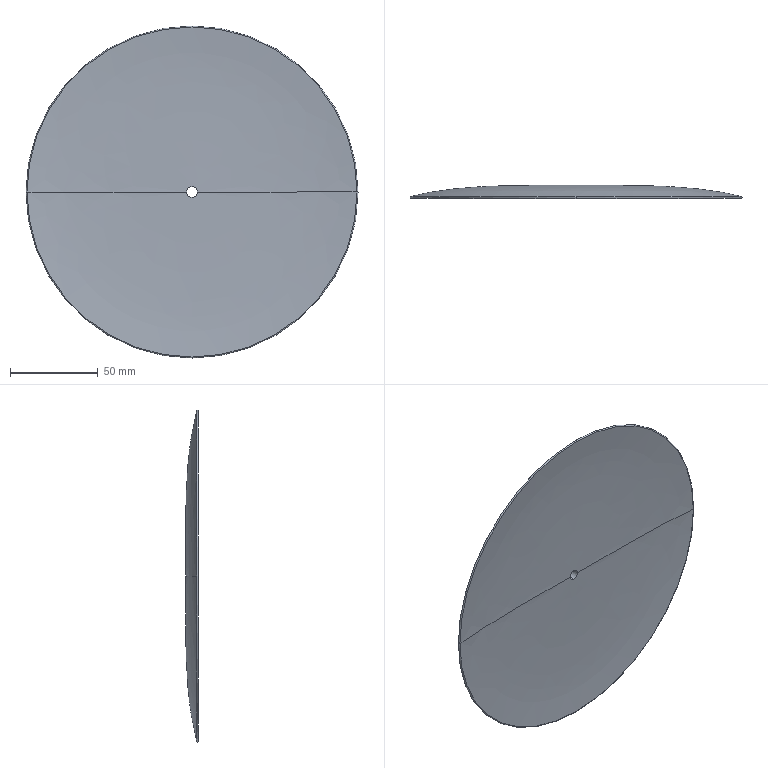Part | SolidWorks | features Fillet 1, ICE 1, Revolution 1 | 1 solid | 8 faces | box 189.61 x 7.325 x 189.61 mm | volume 102683 mm3 | spline 4 | cylinder 2 | torus 2 | commonest cylinder face diameters 6 x2
STEP:
#1=CARTESIAN_POINT('',(0.,-7.131,-94.253));
#2=VERTEX_POINT('',#1);
#3=CARTESIAN_POINT('',(94.253,-7.131,0.));
#4=VERTEX_POINT('',#3);
#5=CARTESIAN_POINT('',(0.,-7.131,0.));
#6=DIRECTION('',(0.,-1.,0.));
#7=DIRECTION('',(0.,0.,1.));
#8=AXIS2_PLACEMENT_3D('',#5,#6,#7);
#9=CIRCLE('',#8,94.253);
#10=EDGE_CURVE('',#2,#4,#9,.T.);
#11=ORIENTED_EDGE('',*,*,#10,.T.);
#12=CARTESIAN_POINT('',(3.,-4.995,0.));
#13=VERTEX_POINT('',#12);
#14=CARTESIAN_POINT('',(94.253,-7.131,0.));
#15=CARTESIAN_POINT('',(66.921,-4.289,0.));
#16=CARTESIAN_POINT('',(24.057,-4.927,0.));
#17=CARTESIAN_POINT('',(3.,-4.995,0.));
#18=B_SPLINE_CURVE_WITH_KNOTS('',3,(#14,#15,#16,#17),.UNSPECIFIED.,.F.,.F.,(4,4),(0.06526,0.9553),.UNSPECIFIED.);
#19=EDGE_CURVE('',#4,#13,#18,.T.);
#20=ORIENTED_EDGE('',*,*,#19,.T.);
#21=CARTESIAN_POINT('',(0.,-4.995,-3.));
#22=VERTEX_POINT('',#21);
#23=CARTESIAN_POINT('',(0.,-4.995,0.));
#24=DIRECTION('',(0.,-1.,0.));
#25=DIRECTION('',(0.,0.,1.));
#26=AXIS2_PLACEMENT_3D('',#23,#24,#25);
#27=CIRCLE('',#26,3.);
#28=EDGE_CURVE('',#22,#13,#27,.T.);
#29=ORIENTED_EDGE('',*,*,#28,.F.);
#30=CARTESIAN_POINT('',(-3.,-4.995,0.));
#31=VERTEX_POINT('',#30);
#32=CARTESIAN_POINT('',(0.,-4.995,0.));
#33=DIRECTION('',(0.,-1.,0.));
#34=DIRECTION('',(0.,0.,1.));
#35=AXIS2_PLACEMENT_3D('',#32,#33,#34);
#36=CIRCLE('',#35,3.);
#37=EDGE_CURVE('',#31,#22,#36,.T.);
#38=ORIENTED_EDGE('',*,*,#37,.F.);
#39=CARTESIAN_POINT('',(-94.253,-7.131,0.));
#40=VERTEX_POINT('',#39);
#41=CARTESIAN_POINT('',(-94.253,-7.131,0.));
#42=CARTESIAN_POINT('',(-66.921,-4.289,0.));
#43=CARTESIAN_POINT('',(-24.057,-4.927,0.));
#44=CARTESIAN_POINT('',(-3.,-4.995,0.));
#45=B_SPLINE_CURVE_WITH_KNOTS('',3,(#41,#42,#43,#44),.UNSPECIFIED.,.F.,.F.,(4,4),(0.06526,0.9553),.UNSPECIFIED.);
#46=EDGE_CURVE('',#40,#31,#45,.T.);
#47=ORIENTED_EDGE('',*,*,#46,.F.);
#48=CARTESIAN_POINT('',(0.,-7.131,0.));
#49=DIRECTION('',(0.,-1.,0.));
#50=DIRECTION('',(0.,0.,1.));
#51=AXIS2_PLACEMENT_3D('',#48,#49,#50);
#52=CIRCLE('',#51,94.253);
#53=EDGE_CURVE('',#40,#2,#52,.T.);
#54=ORIENTED_EDGE('',*,*,#53,.T.);
#55=EDGE_LOOP('',(#11,#20,#29,#38,#47,#54));
#56=FACE_OUTER_BOUND('',#55,.T.);
#57=CARTESIAN_POINT('',(94.253,-7.131,0.));
#58=CARTESIAN_POINT('',(94.253,-7.131,-188.507));
#59=CARTESIAN_POINT('',(-94.253,-7.131,-188.507));
#60=CARTESIAN_POINT('',(-94.253,-7.131,0.));
#61=CARTESIAN_POINT('',(66.921,-4.289,0.));
#62=CARTESIAN_POINT('',(66.921,-4.289,-133.842));
#63=CARTESIAN_POINT('',(-66.921,-4.289,-133.842));
#64=CARTESIAN_POINT('',(-66.921,-4.289,0.));
#65=CARTESIAN_POINT('',(24.057,-4.927,0.));
#66=CARTESIAN_POINT('',(24.057,-4.927,-48.114));
#67=CARTESIAN_POINT('',(-24.057,-4.927,-48.114));
#68=CARTESIAN_POINT('',(-24.057,-4.927,0.));
#69=CARTESIAN_POINT('',(3.,-4.995,0.));
#70=CARTESIAN_POINT('',(3.,-4.995,-6.));
#71=CARTESIAN_POINT('',(-3.,-4.995,-6.));
#72=CARTESIAN_POINT('',(-3.,-4.995,0.));
#73=(BOUNDED_SURFACE()B_SPLINE_SURFACE(3,3,((#57,#58,#59,#60),(#61,#62,#63,#64),(#65,#66,#67,#68),(#69,#70,#71,#72)),.UNSPECIFIED.,.F.,.F.,.F.)B_SPLINE_SURFACE_WITH_KNOTS((4,4),(4,4),(0.06526,0.9553),(0.,1.),.UNSPECIFIED.)GEOMETRIC_REPRESENTATION_ITEM()RATIONAL_B_SPLINE_SURFACE(((1.,0.3333,0.3333,1.),(1.,0.3333,0.3333,1.),(1.,0.3333,0.3333,1.),(1.,0.3333,0.3333,1.)))REPRESENTATION_ITEM('')SURFACE());
#74=ADVANCED_FACE('',(#56),#73,.T.);
#75=CARTESIAN_POINT('',(3.,0.01022,0.));
#76=VERTEX_POINT('',#75);
#77=CARTESIAN_POINT('',(0.,0.01022,-3.));
#78=VERTEX_POINT('',#77);
#79=CARTESIAN_POINT('',(0.,0.01022,0.));
#80=DIRECTION('',(0.,1.,0.));
#81=DIRECTION('',(0.,0.,1.));
#82=AXIS2_PLACEMENT_3D('',#79,#80,#81);
#83=CIRCLE('',#82,3.);
#84=EDGE_CURVE('',#76,#78,#83,.T.);
#85=ORIENTED_EDGE('',*,*,#84,.F.);
#86=CARTESIAN_POINT('',(94.435,-6.151,0.));
#87=VERTEX_POINT('',#86);
#88=CARTESIAN_POINT('',(3.,0.01022,0.));
#89=CARTESIAN_POINT('',(25.237,0.1482,0.));
#90=CARTESIAN_POINT('',(65.845,1.519,0.));
#91=CARTESIAN_POINT('',(94.435,-6.151,0.));
#92=B_SPLINE_CURVE_WITH_KNOTS('',3,(#88,#89,#90,#91),.UNSPECIFIED.,.F.,.F.,(4,4),(0.04205,0.94),.UNSPECIFIED.);
#93=EDGE_CURVE('',#76,#87,#92,.T.);
#94=ORIENTED_EDGE('',*,*,#93,.T.);
#95=CARTESIAN_POINT('',(0.,-6.151,-94.435));
#96=VERTEX_POINT('',#95);
#97=CARTESIAN_POINT('',(0.,-6.151,0.));
#98=DIRECTION('',(0.,1.,0.));
#99=DIRECTION('',(0.,0.,1.));
#100=AXIS2_PLACEMENT_3D('',#97,#98,#99);
#101=CIRCLE('',#100,94.435);
#102=EDGE_CURVE('',#87,#96,#101,.T.);
#103=ORIENTED_EDGE('',*,*,#102,.T.);
#104=CARTESIAN_POINT('',(-94.435,-6.151,0.));
#105=VERTEX_POINT('',#104);
#106=CARTESIAN_POINT('',(0.,-6.151,0.));
#107=DIRECTION('',(0.,1.,0.));
#108=DIRECTION('',(0.,0.,1.));
#109=AXIS2_PLACEMENT_3D('',#106,#107,#108);
#110=CIRCLE('',#109,94.435);
#111=EDGE_CURVE('',#96,#105,#110,.T.);
#112=ORIENTED_EDGE('',*,*,#111,.T.);
#113=CARTESIAN_POINT('',(-3.,0.01022,0.));
#114=VERTEX_POINT('',#113);
#115=CARTESIAN_POINT('',(-3.,0.01022,0.));
#116=CARTESIAN_POINT('',(-25.237,0.1482,0.));
#117=CARTESIAN_POINT('',(-65.845,1.519,0.));
#118=CARTESIAN_POINT('',(-94.435,-6.151,0.));
#119=B_SPLINE_CURVE_WITH_KNOTS('',3,(#115,#116,#117,#118),.UNSPECIFIED.,.F.,.F.,(4,4),(0.04205,0.94),.UNSPECIFIED.);
#120=EDGE_CURVE('',#114,#105,#119,.T.);
#121=ORIENTED_EDGE('',*,*,#120,.F.);
#122=CARTESIAN_POINT('',(0.,0.01022,0.));
#123=DIRECTION('',(0.,1.,0.));
#124=DIRECTION('',(0.,0.,1.));
#125=AXIS2_PLACEMENT_3D('',#122,#123,#124);
#126=CIRCLE('',#125,3.);
#127=EDGE_CURVE('',#78,#114,#126,.T.);
#128=ORIENTED_EDGE('',*,*,#127,.F.);
#129=EDGE_LOOP('',(#85,#94,#103,#112,#121,#128));
#130=FACE_OUTER_BOUND('',#129,.T.);
#131=CARTESIAN_POINT('',(3.,0.01022,0.));
#132=CARTESIAN_POINT('',(3.,0.01022,-6.));
#133=CARTESIAN_POINT('',(-3.,0.01022,-6.));
#134=CARTESIAN_POINT('',(-3.,0.01022,0.));
#135=CARTESIAN_POINT('',(25.237,0.1482,0.));
#136=CARTESIAN_POINT('',(25.237,0.1482,-50.474));
#137=CARTESIAN_POINT('',(-25.237,0.1482,-50.474));
#138=CARTESIAN_POINT('',(-25.237,0.1482,0.));
#139=CARTESIAN_POINT('',(65.845,1.519,0.));
#140=CARTESIAN_POINT('',(65.845,1.519,-131.691));
#141=CARTESIAN_POINT('',(-65.845,1.519,-131.691));
#142=CARTESIAN_POINT('',(-65.845,1.519,0.));
#143=CARTESIAN_POINT('',(94.435,-6.151,0.));
#144=CARTESIAN_POINT('',(94.435,-6.151,-188.869));
#145=CARTESIAN_POINT('',(-94.435,-6.151,-188.869));
#146=CARTESIAN_POINT('',(-94.435,-6.151,0.));
#147=(BOUNDED_SURFACE()B_SPLINE_SURFACE(3,3,((#131,#132,#133,#134),(#135,#136,#137,#138),(#139,#140,#141,#142),(#143,#144,#145,#146)),.UNSPECIFIED.,.F.,.F.,.F.)B_SPLINE_SURFACE_WITH_KNOTS((4,4),(4,4),(0.04205,0.94),(0.,1.),.UNSPECIFIED.)GEOMETRIC_REPRESENTATION_ITEM()RATIONAL_B_SPLINE_SURFACE(((1.,0.3333,0.3333,1.),(1.,0.3333,0.3333,1.),(1.,0.3333,0.3333,1.),(1.,0.3333,0.3333,1.)))REPRESENTATION_ITEM('')SURFACE());
#148=ADVANCED_FACE('',(#130),#147,.T.);
#149=CARTESIAN_POINT('',(0.,-4.995,3.));
#150=VERTEX_POINT('',#149);
#151=CARTESIAN_POINT('',(0.,-4.995,0.));
#152=DIRECTION('',(0.,-1.,0.));
#153=DIRECTION('',(0.,0.,1.));
#154=AXIS2_PLACEMENT_3D('',#151,#152,#153);
#155=CIRCLE('',#154,3.);
#156=EDGE_CURVE('',#150,#31,#155,.T.);
#157=ORIENTED_EDGE('',*,*,#156,.T.);
#158=ORIENTED_EDGE('',*,*,#37,.T.);
#159=CARTESIAN_POINT('',(0.,-23.,-3.));
#160=DIRECTION('',(0.,1.,0.));
#161=VECTOR('',#160,1000.);
#162=LINE('',#159,#161);
#163=EDGE_CURVE('',#22,#78,#162,.T.);
#164=ORIENTED_EDGE('',*,*,#163,.T.);
#165=ORIENTED_EDGE('',*,*,#127,.T.);
#166=CARTESIAN_POINT('',(0.,0.01022,3.));
#167=VERTEX_POINT('',#166);
#168=CARTESIAN_POINT('',(0.,0.01022,0.));
#169=DIRECTION('',(0.,1.,0.));
#170=DIRECTION('',(0.,0.,1.));
#171=AXIS2_PLACEMENT_3D('',#168,#169,#170);
#172=CIRCLE('',#171,3.);
#173=EDGE_CURVE('',#114,#167,#172,.T.);
#174=ORIENTED_EDGE('',*,*,#173,.T.);
#175=CARTESIAN_POINT('',(0.,-23.,3.));
#176=DIRECTION('',(0.,1.,0.));
#177=VECTOR('',#176,1000.);
#178=LINE('',#175,#177);
#179=EDGE_CURVE('',#150,#167,#178,.T.);
#180=ORIENTED_EDGE('',*,*,#179,.F.);
#181=EDGE_LOOP('',(#157,#158,#164,#165,#174,#180));
#182=FACE_OUTER_BOUND('',#181,.T.);
#183=CARTESIAN_POINT('',(0.,-23.,0.));
#184=DIRECTION('',(0.,1.,0.));
#185=DIRECTION('',(0.,0.,1.));
#186=AXIS2_PLACEMENT_3D('',#183,#184,#185);
#187=CYLINDRICAL_SURFACE('',#186,3.);
#188=ADVANCED_FACE('',(#182),#187,.F.);
#189=CARTESIAN_POINT('',(0.,-6.151,94.435));
#190=VERTEX_POINT('',#189);
#191=CARTESIAN_POINT('',(0.,-6.151,0.));
#192=DIRECTION('',(0.,1.,0.));
#193=DIRECTION('',(0.,0.,1.));
#194=AXIS2_PLACEMENT_3D('',#191,#192,#193);
#195=CIRCLE('',#194,94.435);
#196=EDGE_CURVE('',#190,#87,#195,.T.);
#197=ORIENTED_EDGE('',*,*,#196,.F.);
#198=CARTESIAN_POINT('',(0.,-7.131,94.253));
#199=VERTEX_POINT('',#198);
#200=CARTESIAN_POINT('',(0.,-6.634,94.305));
#201=DIRECTION('',(1.,0.,0.));
#202=DIRECTION('',(0.,0.,-1.));
#203=AXIS2_PLACEMENT_3D('',#200,#201,#202);
#204=CIRCLE('',#203,0.5);
#205=EDGE_CURVE('',#190,#199,#204,.T.);
#206=ORIENTED_EDGE('',*,*,#205,.T.);
#207=CARTESIAN_POINT('',(0.,-7.131,0.));
#208=DIRECTION('',(0.,-1.,0.));
#209=DIRECTION('',(0.,0.,1.));
#210=AXIS2_PLACEMENT_3D('',#207,#208,#209);
#211=CIRCLE('',#210,94.253);
#212=EDGE_CURVE('',#4,#199,#211,.T.);
#213=ORIENTED_EDGE('',*,*,#212,.F.);
#214=ORIENTED_EDGE('',*,*,#10,.F.);
#215=CARTESIAN_POINT('',(0.,-6.634,-94.305));
#216=DIRECTION('',(-1.,0.,0.));
#217=DIRECTION('',(0.,0.,1.));
#218=AXIS2_PLACEMENT_3D('',#215,#216,#217);
#219=CIRCLE('',#218,0.5);
#220=EDGE_CURVE('',#96,#2,#219,.T.);
#221=ORIENTED_EDGE('',*,*,#220,.F.);
#222=ORIENTED_EDGE('',*,*,#102,.F.);
#223=EDGE_LOOP('',(#197,#206,#213,#214,#221,#222));
#224=FACE_OUTER_BOUND('',#223,.T.);
#225=CARTESIAN_POINT('',(0.,-6.634,0.));
#226=DIRECTION('',(0.,-1.,0.));
#227=DIRECTION('',(0.,0.,-1.));
#228=AXIS2_PLACEMENT_3D('',#225,#226,#227);
#229=TOROIDAL_SURFACE('',#228,94.305,0.5);
#230=ADVANCED_FACE('',(#224),#229,.T.);
#231=ORIENTED_EDGE('',*,*,#93,.F.);
#232=CARTESIAN_POINT('',(0.,0.01022,0.));
#233=DIRECTION('',(0.,1.,0.));
#234=DIRECTION('',(0.,0.,1.));
#235=AXIS2_PLACEMENT_3D('',#232,#233,#234);
#236=CIRCLE('',#235,3.);
#237=EDGE_CURVE('',#167,#76,#236,.T.);
#238=ORIENTED_EDGE('',*,*,#237,.F.);
#239=ORIENTED_EDGE('',*,*,#173,.F.);
#240=ORIENTED_EDGE('',*,*,#120,.T.);
#241=CARTESIAN_POINT('',(0.,-6.151,0.));
#242=DIRECTION('',(0.,1.,0.));
#243=DIRECTION('',(0.,0.,1.));
#244=AXIS2_PLACEMENT_3D('',#241,#242,#243);
#245=CIRCLE('',#244,94.435);
#246=EDGE_CURVE('',#105,#190,#245,.T.);
#247=ORIENTED_EDGE('',*,*,#246,.T.);
#248=ORIENTED_EDGE('',*,*,#196,.T.);
#249=EDGE_LOOP('',(#231,#238,#239,#240,#247,#248));
#250=FACE_OUTER_BOUND('',#249,.T.);
#251=CARTESIAN_POINT('',(-3.,0.01022,0.));
#252=CARTESIAN_POINT('',(-3.,0.01022,6.));
#253=CARTESIAN_POINT('',(3.,0.01022,6.));
#254=CARTESIAN_POINT('',(3.,0.01022,0.));
#255=CARTESIAN_POINT('',(-25.237,0.1482,0.));
#256=CARTESIAN_POINT('',(-25.237,0.1482,50.474));
#257=CARTESIAN_POINT('',(25.237,0.1482,50.474));
#258=CARTESIAN_POINT('',(25.237,0.1482,0.));
#259=CARTESIAN_POINT('',(-65.845,1.519,0.));
#260=CARTESIAN_POINT('',(-65.845,1.519,131.691));
#261=CARTESIAN_POINT('',(65.845,1.519,131.691));
#262=CARTESIAN_POINT('',(65.845,1.519,0.));
#263=CARTESIAN_POINT('',(-94.435,-6.151,0.));
#264=CARTESIAN_POINT('',(-94.435,-6.151,188.869));
#265=CARTESIAN_POINT('',(94.435,-6.151,188.869));
#266=CARTESIAN_POINT('',(94.435,-6.151,0.));
#267=(BOUNDED_SURFACE()B_SPLINE_SURFACE(3,3,((#251,#252,#253,#254),(#255,#256,#257,#258),(#259,#260,#261,#262),(#263,#264,#265,#266)),.UNSPECIFIED.,.F.,.F.,.F.)B_SPLINE_SURFACE_WITH_KNOTS((4,4),(4,4),(0.04205,0.94),(0.,1.),.UNSPECIFIED.)GEOMETRIC_REPRESENTATION_ITEM()RATIONAL_B_SPLINE_SURFACE(((1.,0.3333,0.3333,1.),(1.,0.3333,0.3333,1.),(1.,0.3333,0.3333,1.),(1.,0.3333,0.3333,1.)))REPRESENTATION_ITEM('')SURFACE());
#268=ADVANCED_FACE('',(#250),#267,.T.);
#269=ORIENTED_EDGE('',*,*,#19,.F.);
#270=ORIENTED_EDGE('',*,*,#212,.T.);
#271=CARTESIAN_POINT('',(0.,-7.131,0.));
#272=DIRECTION('',(0.,-1.,0.));
#273=DIRECTION('',(0.,0.,1.));
#274=AXIS2_PLACEMENT_3D('',#271,#272,#273);
#275=CIRCLE('',#274,94.253);
#276=EDGE_CURVE('',#199,#40,#275,.T.);
#277=ORIENTED_EDGE('',*,*,#276,.T.);
#278=ORIENTED_EDGE('',*,*,#46,.T.);
#279=ORIENTED_EDGE('',*,*,#156,.F.);
#280=CARTESIAN_POINT('',(0.,-4.995,0.));
#281=DIRECTION('',(0.,-1.,0.));
#282=DIRECTION('',(0.,0.,1.));
#283=AXIS2_PLACEMENT_3D('',#280,#281,#282);
#284=CIRCLE('',#283,3.);
#285=EDGE_CURVE('',#13,#150,#284,.T.);
#286=ORIENTED_EDGE('',*,*,#285,.F.);
#287=EDGE_LOOP('',(#269,#270,#277,#278,#279,#286));
#288=FACE_OUTER_BOUND('',#287,.T.);
#289=CARTESIAN_POINT('',(-94.253,-7.131,0.));
#290=CARTESIAN_POINT('',(-94.253,-7.131,188.507));
#291=CARTESIAN_POINT('',(94.253,-7.131,188.507));
#292=CARTESIAN_POINT('',(94.253,-7.131,0.));
#293=CARTESIAN_POINT('',(-66.921,-4.289,0.));
#294=CARTESIAN_POINT('',(-66.921,-4.289,133.842));
#295=CARTESIAN_POINT('',(66.921,-4.289,133.842));
#296=CARTESIAN_POINT('',(66.921,-4.289,0.));
#297=CARTESIAN_POINT('',(-24.057,-4.927,0.));
#298=CARTESIAN_POINT('',(-24.057,-4.927,48.114));
#299=CARTESIAN_POINT('',(24.057,-4.927,48.114));
#300=CARTESIAN_POINT('',(24.057,-4.927,0.));
#301=CARTESIAN_POINT('',(-3.,-4.995,0.));
#302=CARTESIAN_POINT('',(-3.,-4.995,6.));
#303=CARTESIAN_POINT('',(3.,-4.995,6.));
#304=CARTESIAN_POINT('',(3.,-4.995,0.));
#305=(BOUNDED_SURFACE()B_SPLINE_SURFACE(3,3,((#289,#290,#291,#292),(#293,#294,#295,#296),(#297,#298,#299,#300),(#301,#302,#303,#304)),.UNSPECIFIED.,.F.,.F.,.F.)B_SPLINE_SURFACE_WITH_KNOTS((4,4),(4,4),(0.06526,0.9553),(0.,1.),.UNSPECIFIED.)GEOMETRIC_REPRESENTATION_ITEM()RATIONAL_B_SPLINE_SURFACE(((1.,0.3333,0.3333,1.),(1.,0.3333,0.3333,1.),(1.,0.3333,0.3333,1.),(1.,0.3333,0.3333,1.)))REPRESENTATION_ITEM('')SURFACE());
#306=ADVANCED_FACE('',(#288),#305,.T.);
#307=ORIENTED_EDGE('',*,*,#205,.F.);
#308=ORIENTED_EDGE('',*,*,#246,.F.);
#309=ORIENTED_EDGE('',*,*,#111,.F.);
#310=ORIENTED_EDGE('',*,*,#220,.T.);
#311=ORIENTED_EDGE('',*,*,#53,.F.);
#312=ORIENTED_EDGE('',*,*,#276,.F.);
#313=EDGE_LOOP('',(#307,#308,#309,#310,#311,#312));
#314=FACE_OUTER_BOUND('',#313,.T.);
#315=CARTESIAN_POINT('',(0.,-6.634,0.));
#316=DIRECTION('',(0.,-1.,0.));
#317=DIRECTION('',(0.,0.,-1.));
#318=AXIS2_PLACEMENT_3D('',#315,#316,#317);
#319=TOROIDAL_SURFACE('',#318,94.305,0.5);
#320=ADVANCED_FACE('',(#314),#319,.T.);
#321=ORIENTED_EDGE('',*,*,#163,.F.);
#322=ORIENTED_EDGE('',*,*,#28,.T.);
#323=ORIENTED_EDGE('',*,*,#285,.T.);
#324=ORIENTED_EDGE('',*,*,#179,.T.);
#325=ORIENTED_EDGE('',*,*,#237,.T.);
#326=ORIENTED_EDGE('',*,*,#84,.T.);
#327=EDGE_LOOP('',(#321,#322,#323,#324,#325,#326));
#328=FACE_OUTER_BOUND('',#327,.T.);
#329=CARTESIAN_POINT('',(0.,-23.,0.));
#330=DIRECTION('',(0.,1.,0.));
#331=DIRECTION('',(0.,0.,1.));
#332=AXIS2_PLACEMENT_3D('',#329,#330,#331);
#333=CYLINDRICAL_SURFACE('',#332,3.);
#334=ADVANCED_FACE('',(#328),#333,.F.);
#335=CLOSED_SHELL('',(#74,#148,#188,#230,#268,#306,#320,#334));
#336=MANIFOLD_SOLID_BREP('',#335);
#337=CARTESIAN_POINT('',(0.,0.,0.));
#338=DIRECTION('',(0.,0.,1.));
#339=DIRECTION('',(1.,0.,0.));
#340=AXIS2_PLACEMENT_3D('',#337,#338,#339);
#341=(LENGTH_UNIT()NAMED_UNIT(*)SI_UNIT(.MILLI.,.METRE.));
#342=UNCERTAINTY_MEASURE_WITH_UNIT(LENGTH_MEASURE(0.00001),#341,'','');
#343=(NAMED_UNIT(*)PLANE_ANGLE_UNIT()SI_UNIT($,.RADIAN.));
#344=(NAMED_UNIT(*)SI_UNIT($,.STERADIAN.)SOLID_ANGLE_UNIT());
#345=(GEOMETRIC_REPRESENTATION_CONTEXT(3)GLOBAL_UNCERTAINTY_ASSIGNED_CONTEXT((#342))GLOBAL_UNIT_ASSIGNED_CONTEXT((#341,#343,#344))REPRESENTATION_CONTEXT('',''));
#346=ADVANCED_BREP_SHAPE_REPRESENTATION('',(#336,#340),#345);